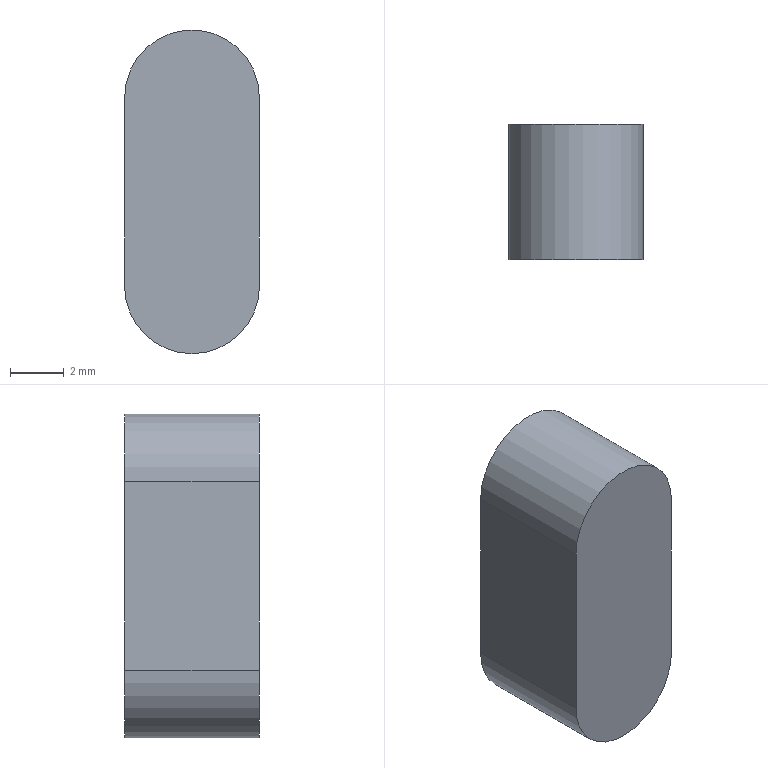Part | STEP file | BLC03-B5-L12 | 1 solid | 7 faces | box 5 x 5 x 12 mm | volume 273.175 mm3 | plane 4 | cylinder 3 | commonest cylinder face diameters 5 x3
STEP:
#1=CARTESIAN_POINT('',(0.,0.,0.));
#2=DIRECTION('',(0.,0.,1.));
#3=DIRECTION('',(1.,0.,0.));
#4=AXIS2_PLACEMENT_3D('',#1,#2,#3);
#5=CARTESIAN_POINT('',(0.,2.5,-6.));
#6=VERTEX_POINT('',#5);
#7=CARTESIAN_POINT('',(-2.5,2.5,-3.5));
#8=VERTEX_POINT('',#7);
#9=CARTESIAN_POINT('',(0.,2.5,-3.5));
#10=DIRECTION('',(0.,1.,0.));
#11=DIRECTION('',(0.,0.,1.));
#12=AXIS2_PLACEMENT_3D('',#9,#10,#11);
#13=CIRCLE('',#12,2.5);
#14=CARTESIAN_POINT('',(0.,2.5,-3.5));
#15=DIRECTION('',(0.,-1.,0.));
#16=DIRECTION('',(0.,0.,-1.));
#17=AXIS2_PLACEMENT_3D('',#14,#15,#16);
#18=CYLINDRICAL_SURFACE('',#17,2.5);
#19=CARTESIAN_POINT('',(9.425,0.));
#20=DIRECTION('',(-1.,0.));
#21=VECTOR('',#20,1.);
#22=LINE('',#19,#21);
#23=(GEOMETRIC_REPRESENTATION_CONTEXT(2)PARAMETRIC_REPRESENTATION_CONTEXT()REPRESENTATION_CONTEXT('',''));
#24=DEFINITIONAL_REPRESENTATION('',(#22),#23);
#25=PCURVE('',#18,#24);
#26=CARTESIAN_POINT('',(0.,2.5,3.5));
#27=DIRECTION('',(0.,1.,0.));
#28=DIRECTION('',(0.,0.,1.));
#29=AXIS2_PLACEMENT_3D('',#26,#27,#28);
#30=PLANE('',#29);
#31=CARTESIAN_POINT('',(-7.,0.));
#32=DIRECTION('',(1.,0.));
#33=AXIS2_PLACEMENT_2D('',#31,#32);
#34=CIRCLE('',#33,2.5);
#35=(GEOMETRIC_REPRESENTATION_CONTEXT(2)PARAMETRIC_REPRESENTATION_CONTEXT()REPRESENTATION_CONTEXT('',''));
#36=DEFINITIONAL_REPRESENTATION('',(#34),#35);
#37=PCURVE('',#30,#36);
#38=SURFACE_CURVE('',#13,(#25,#37),.PCURVE_S1.);
#39=EDGE_CURVE('',#6,#8,#38,.T.);
#40=ORIENTED_EDGE('',*,*,#39,.F.);
#41=CARTESIAN_POINT('',(0.,-2.5,-6.));
#42=VERTEX_POINT('',#41);
#43=CARTESIAN_POINT('',(0.,2.5,-6.));
#44=DIRECTION('',(0.,-1.,0.));
#45=VECTOR('',#44,1.);
#46=LINE('',#43,#45);
#47=CARTESIAN_POINT('',(6.283,0.));
#48=DIRECTION('',(0.,1.));
#49=VECTOR('',#48,1.);
#50=LINE('',#47,#49);
#51=(GEOMETRIC_REPRESENTATION_CONTEXT(2)PARAMETRIC_REPRESENTATION_CONTEXT()REPRESENTATION_CONTEXT('',''));
#52=DEFINITIONAL_REPRESENTATION('',(#50),#51);
#53=PCURVE('',#18,#52);
#54=CARTESIAN_POINT('',(0.,2.5,-3.5));
#55=DIRECTION('',(0.,-1.,0.));
#56=DIRECTION('',(0.,0.,-1.));
#57=AXIS2_PLACEMENT_3D('',#54,#55,#56);
#58=CYLINDRICAL_SURFACE('',#57,2.5);
#59=CARTESIAN_POINT('',(0.,0.));
#60=DIRECTION('',(0.,1.));
#61=VECTOR('',#60,1.);
#62=LINE('',#59,#61);
#63=(GEOMETRIC_REPRESENTATION_CONTEXT(2)PARAMETRIC_REPRESENTATION_CONTEXT()REPRESENTATION_CONTEXT('',''));
#64=DEFINITIONAL_REPRESENTATION('',(#62),#63);
#65=PCURVE('',#58,#64);
#66=SURFACE_CURVE('',#46,(#53,#65),.PCURVE_S1.);
#67=EDGE_CURVE('',#6,#42,#66,.T.);
#68=ORIENTED_EDGE('',*,*,#67,.T.);
#69=CARTESIAN_POINT('',(-2.5,-2.5,-3.5));
#70=VERTEX_POINT('',#69);
#71=CARTESIAN_POINT('',(0.,-2.5,-3.5));
#72=DIRECTION('',(0.,1.,0.));
#73=DIRECTION('',(0.,0.,1.));
#74=AXIS2_PLACEMENT_3D('',#71,#72,#73);
#75=CIRCLE('',#74,2.5);
#76=CARTESIAN_POINT('',(9.425,5.));
#77=DIRECTION('',(-1.,0.));
#78=VECTOR('',#77,1.);
#79=LINE('',#76,#78);
#80=(GEOMETRIC_REPRESENTATION_CONTEXT(2)PARAMETRIC_REPRESENTATION_CONTEXT()REPRESENTATION_CONTEXT('',''));
#81=DEFINITIONAL_REPRESENTATION('',(#79),#80);
#82=PCURVE('',#18,#81);
#83=CARTESIAN_POINT('',(0.,-2.5,3.5));
#84=DIRECTION('',(0.,1.,0.));
#85=DIRECTION('',(0.,0.,1.));
#86=AXIS2_PLACEMENT_3D('',#83,#84,#85);
#87=PLANE('',#86);
#88=CARTESIAN_POINT('',(-7.,0.));
#89=DIRECTION('',(1.,0.));
#90=AXIS2_PLACEMENT_2D('',#88,#89);
#91=CIRCLE('',#90,2.5);
#92=(GEOMETRIC_REPRESENTATION_CONTEXT(2)PARAMETRIC_REPRESENTATION_CONTEXT()REPRESENTATION_CONTEXT('',''));
#93=DEFINITIONAL_REPRESENTATION('',(#91),#92);
#94=PCURVE('',#87,#93);
#95=SURFACE_CURVE('',#75,(#82,#94),.PCURVE_S1.);
#96=EDGE_CURVE('',#42,#70,#95,.T.);
#97=ORIENTED_EDGE('',*,*,#96,.T.);
#98=CARTESIAN_POINT('',(-2.5,2.5,-3.5));
#99=DIRECTION('',(0.,-1.,0.));
#100=VECTOR('',#99,1.);
#101=LINE('',#98,#100);
#102=CARTESIAN_POINT('',(4.712,0.));
#103=DIRECTION('',(0.,1.));
#104=VECTOR('',#103,1.);
#105=LINE('',#102,#104);
#106=(GEOMETRIC_REPRESENTATION_CONTEXT(2)PARAMETRIC_REPRESENTATION_CONTEXT()REPRESENTATION_CONTEXT('',''));
#107=DEFINITIONAL_REPRESENTATION('',(#105),#106);
#108=PCURVE('',#18,#107);
#109=CARTESIAN_POINT('',(-2.5,2.5,-3.5));
#110=DIRECTION('',(1.,0.,0.));
#111=DIRECTION('',(0.,0.,-1.));
#112=AXIS2_PLACEMENT_3D('',#109,#110,#111);
#113=PLANE('',#112);
#114=CARTESIAN_POINT('',(0.,0.));
#115=DIRECTION('',(0.,-1.));
#116=VECTOR('',#115,1.);
#117=LINE('',#114,#116);
#118=(GEOMETRIC_REPRESENTATION_CONTEXT(2)PARAMETRIC_REPRESENTATION_CONTEXT()REPRESENTATION_CONTEXT('',''));
#119=DEFINITIONAL_REPRESENTATION('',(#117),#118);
#120=PCURVE('',#113,#119);
#121=SURFACE_CURVE('',#101,(#108,#120),.PCURVE_S1.);
#122=EDGE_CURVE('',#8,#70,#121,.T.);
#123=ORIENTED_EDGE('',*,*,#122,.F.);
#124=EDGE_LOOP('',(#40,#68,#97,#123));
#125=FACE_BOUND('',#124,.T.);
#126=ADVANCED_FACE('',(#125),#18,.T.);
#127=CARTESIAN_POINT('',(2.5,-2.5,-3.5));
#128=VERTEX_POINT('',#127);
#129=CARTESIAN_POINT('',(2.5,-2.5,3.5));
#130=VERTEX_POINT('',#129);
#131=CARTESIAN_POINT('',(2.5,-2.5,-3.5));
#132=DIRECTION('',(0.,0.,1.));
#133=VECTOR('',#132,1.);
#134=LINE('',#131,#133);
#135=CARTESIAN_POINT('',(2.5,2.5,-3.5));
#136=DIRECTION('',(1.,0.,0.));
#137=DIRECTION('',(0.,0.,-1.));
#138=AXIS2_PLACEMENT_3D('',#135,#136,#137);
#139=PLANE('',#138);
#140=CARTESIAN_POINT('',(0.,-5.));
#141=DIRECTION('',(-1.,0.));
#142=VECTOR('',#141,1.);
#143=LINE('',#140,#142);
#144=(GEOMETRIC_REPRESENTATION_CONTEXT(2)PARAMETRIC_REPRESENTATION_CONTEXT()REPRESENTATION_CONTEXT('',''));
#145=DEFINITIONAL_REPRESENTATION('',(#143),#144);
#146=PCURVE('',#139,#145);
#147=CARTESIAN_POINT('',(-7.,2.5));
#148=DIRECTION('',(1.,0.));
#149=VECTOR('',#148,1.);
#150=LINE('',#147,#149);
#151=(GEOMETRIC_REPRESENTATION_CONTEXT(2)PARAMETRIC_REPRESENTATION_CONTEXT()REPRESENTATION_CONTEXT('',''));
#152=DEFINITIONAL_REPRESENTATION('',(#150),#151);
#153=PCURVE('',#87,#152);
#154=SURFACE_CURVE('',#134,(#146,#153),.PCURVE_S1.);
#155=EDGE_CURVE('',#128,#130,#154,.T.);
#156=ORIENTED_EDGE('',*,*,#155,.F.);
#157=CARTESIAN_POINT('',(2.5,2.5,-3.5));
#158=VERTEX_POINT('',#157);
#159=CARTESIAN_POINT('',(2.5,2.5,-3.5));
#160=DIRECTION('',(0.,-1.,0.));
#161=VECTOR('',#160,1.);
#162=LINE('',#159,#161);
#163=CARTESIAN_POINT('',(0.,0.));
#164=DIRECTION('',(0.,-1.));
#165=VECTOR('',#164,1.);
#166=LINE('',#163,#165);
#167=(GEOMETRIC_REPRESENTATION_CONTEXT(2)PARAMETRIC_REPRESENTATION_CONTEXT()REPRESENTATION_CONTEXT('',''));
#168=DEFINITIONAL_REPRESENTATION('',(#166),#167);
#169=PCURVE('',#139,#168);
#170=CARTESIAN_POINT('',(1.571,0.));
#171=DIRECTION('',(0.,1.));
#172=VECTOR('',#171,1.);
#173=LINE('',#170,#172);
#174=(GEOMETRIC_REPRESENTATION_CONTEXT(2)PARAMETRIC_REPRESENTATION_CONTEXT()REPRESENTATION_CONTEXT('',''));
#175=DEFINITIONAL_REPRESENTATION('',(#173),#174);
#176=PCURVE('',#58,#175);
#177=SURFACE_CURVE('',#162,(#169,#176),.PCURVE_S1.);
#178=EDGE_CURVE('',#158,#128,#177,.T.);
#179=ORIENTED_EDGE('',*,*,#178,.F.);
#180=CARTESIAN_POINT('',(2.5,2.5,3.5));
#181=VERTEX_POINT('',#180);
#182=CARTESIAN_POINT('',(2.5,2.5,-3.5));
#183=DIRECTION('',(0.,0.,1.));
#184=VECTOR('',#183,1.);
#185=LINE('',#182,#184);
#186=CARTESIAN_POINT('',(0.,0.));
#187=DIRECTION('',(-1.,0.));
#188=VECTOR('',#187,1.);
#189=LINE('',#186,#188);
#190=(GEOMETRIC_REPRESENTATION_CONTEXT(2)PARAMETRIC_REPRESENTATION_CONTEXT()REPRESENTATION_CONTEXT('',''));
#191=DEFINITIONAL_REPRESENTATION('',(#189),#190);
#192=PCURVE('',#139,#191);
#193=CARTESIAN_POINT('',(-7.,2.5));
#194=DIRECTION('',(1.,0.));
#195=VECTOR('',#194,1.);
#196=LINE('',#193,#195);
#197=(GEOMETRIC_REPRESENTATION_CONTEXT(2)PARAMETRIC_REPRESENTATION_CONTEXT()REPRESENTATION_CONTEXT('',''));
#198=DEFINITIONAL_REPRESENTATION('',(#196),#197);
#199=PCURVE('',#30,#198);
#200=SURFACE_CURVE('',#185,(#192,#199),.PCURVE_S1.);
#201=EDGE_CURVE('',#158,#181,#200,.T.);
#202=ORIENTED_EDGE('',*,*,#201,.T.);
#203=CARTESIAN_POINT('',(2.5,2.5,3.5));
#204=DIRECTION('',(0.,-1.,0.));
#205=VECTOR('',#204,1.);
#206=LINE('',#203,#205);
#207=CARTESIAN_POINT('',(-7.,0.));
#208=DIRECTION('',(0.,-1.));
#209=VECTOR('',#208,1.);
#210=LINE('',#207,#209);
#211=(GEOMETRIC_REPRESENTATION_CONTEXT(2)PARAMETRIC_REPRESENTATION_CONTEXT()REPRESENTATION_CONTEXT('',''));
#212=DEFINITIONAL_REPRESENTATION('',(#210),#211);
#213=PCURVE('',#139,#212);
#214=CARTESIAN_POINT('',(0.,2.5,3.5));
#215=DIRECTION('',(0.,-1.,0.));
#216=DIRECTION('',(0.,0.,-1.));
#217=AXIS2_PLACEMENT_3D('',#214,#215,#216);
#218=CYLINDRICAL_SURFACE('',#217,2.5);
#219=CARTESIAN_POINT('',(1.571,0.));
#220=DIRECTION('',(0.,1.));
#221=VECTOR('',#220,1.);
#222=LINE('',#219,#221);
#223=(GEOMETRIC_REPRESENTATION_CONTEXT(2)PARAMETRIC_REPRESENTATION_CONTEXT()REPRESENTATION_CONTEXT('',''));
#224=DEFINITIONAL_REPRESENTATION('',(#222),#223);
#225=PCURVE('',#218,#224);
#226=SURFACE_CURVE('',#206,(#213,#225),.PCURVE_S1.);
#227=EDGE_CURVE('',#181,#130,#226,.T.);
#228=ORIENTED_EDGE('',*,*,#227,.T.);
#229=EDGE_LOOP('',(#156,#179,#202,#228));
#230=FACE_BOUND('',#229,.T.);
#231=ADVANCED_FACE('',(#230),#139,.T.);
#232=ORIENTED_EDGE('',*,*,#67,.F.);
#233=CARTESIAN_POINT('',(0.,2.5,-3.5));
#234=DIRECTION('',(0.,1.,0.));
#235=DIRECTION('',(0.,0.,1.));
#236=AXIS2_PLACEMENT_3D('',#233,#234,#235);
#237=CIRCLE('',#236,2.5);
#238=CARTESIAN_POINT('',(3.142,0.));
#239=DIRECTION('',(-1.,0.));
#240=VECTOR('',#239,1.);
#241=LINE('',#238,#240);
#242=(GEOMETRIC_REPRESENTATION_CONTEXT(2)PARAMETRIC_REPRESENTATION_CONTEXT()REPRESENTATION_CONTEXT('',''));
#243=DEFINITIONAL_REPRESENTATION('',(#241),#242);
#244=PCURVE('',#58,#243);
#245=CARTESIAN_POINT('',(-7.,0.));
#246=DIRECTION('',(1.,0.));
#247=AXIS2_PLACEMENT_2D('',#245,#246);
#248=CIRCLE('',#247,2.5);
#249=(GEOMETRIC_REPRESENTATION_CONTEXT(2)PARAMETRIC_REPRESENTATION_CONTEXT()REPRESENTATION_CONTEXT('',''));
#250=DEFINITIONAL_REPRESENTATION('',(#248),#249);
#251=PCURVE('',#30,#250);
#252=SURFACE_CURVE('',#237,(#244,#251),.PCURVE_S1.);
#253=EDGE_CURVE('',#158,#6,#252,.T.);
#254=ORIENTED_EDGE('',*,*,#253,.F.);
#255=ORIENTED_EDGE('',*,*,#178,.T.);
#256=CARTESIAN_POINT('',(0.,-2.5,-3.5));
#257=DIRECTION('',(0.,1.,0.));
#258=DIRECTION('',(0.,0.,1.));
#259=AXIS2_PLACEMENT_3D('',#256,#257,#258);
#260=CIRCLE('',#259,2.5);
#261=CARTESIAN_POINT('',(3.142,5.));
#262=DIRECTION('',(-1.,0.));
#263=VECTOR('',#262,1.);
#264=LINE('',#261,#263);
#265=(GEOMETRIC_REPRESENTATION_CONTEXT(2)PARAMETRIC_REPRESENTATION_CONTEXT()REPRESENTATION_CONTEXT('',''));
#266=DEFINITIONAL_REPRESENTATION('',(#264),#265);
#267=PCURVE('',#58,#266);
#268=CARTESIAN_POINT('',(-7.,0.));
#269=DIRECTION('',(1.,0.));
#270=AXIS2_PLACEMENT_2D('',#268,#269);
#271=CIRCLE('',#270,2.5);
#272=(GEOMETRIC_REPRESENTATION_CONTEXT(2)PARAMETRIC_REPRESENTATION_CONTEXT()REPRESENTATION_CONTEXT('',''));
#273=DEFINITIONAL_REPRESENTATION('',(#271),#272);
#274=PCURVE('',#87,#273);
#275=SURFACE_CURVE('',#260,(#267,#274),.PCURVE_S1.);
#276=EDGE_CURVE('',#128,#42,#275,.T.);
#277=ORIENTED_EDGE('',*,*,#276,.T.);
#278=EDGE_LOOP('',(#232,#254,#255,#277));
#279=FACE_BOUND('',#278,.T.);
#280=ADVANCED_FACE('',(#279),#58,.T.);
#281=CARTESIAN_POINT('',(-2.5,-2.5,3.5));
#282=VERTEX_POINT('',#281);
#283=CARTESIAN_POINT('',(-2.5,-2.5,-3.5));
#284=DIRECTION('',(0.,0.,1.));
#285=VECTOR('',#284,1.);
#286=LINE('',#283,#285);
#287=CARTESIAN_POINT('',(0.,-5.));
#288=DIRECTION('',(-1.,0.));
#289=VECTOR('',#288,1.);
#290=LINE('',#287,#289);
#291=(GEOMETRIC_REPRESENTATION_CONTEXT(2)PARAMETRIC_REPRESENTATION_CONTEXT()REPRESENTATION_CONTEXT('',''));
#292=DEFINITIONAL_REPRESENTATION('',(#290),#291);
#293=PCURVE('',#113,#292);
#294=CARTESIAN_POINT('',(-7.,-2.5));
#295=DIRECTION('',(1.,0.));
#296=VECTOR('',#295,1.);
#297=LINE('',#294,#296);
#298=(GEOMETRIC_REPRESENTATION_CONTEXT(2)PARAMETRIC_REPRESENTATION_CONTEXT()REPRESENTATION_CONTEXT('',''));
#299=DEFINITIONAL_REPRESENTATION('',(#297),#298);
#300=PCURVE('',#87,#299);
#301=SURFACE_CURVE('',#286,(#293,#300),.PCURVE_S1.);
#302=EDGE_CURVE('',#70,#282,#301,.T.);
#303=ORIENTED_EDGE('',*,*,#302,.T.);
#304=CARTESIAN_POINT('',(-2.5,2.5,3.5));
#305=VERTEX_POINT('',#304);
#306=CARTESIAN_POINT('',(-2.5,2.5,3.5));
#307=DIRECTION('',(0.,-1.,0.));
#308=VECTOR('',#307,1.);
#309=LINE('',#306,#308);
#310=CARTESIAN_POINT('',(-7.,0.));
#311=DIRECTION('',(0.,-1.));
#312=VECTOR('',#311,1.);
#313=LINE('',#310,#312);
#314=(GEOMETRIC_REPRESENTATION_CONTEXT(2)PARAMETRIC_REPRESENTATION_CONTEXT()REPRESENTATION_CONTEXT('',''));
#315=DEFINITIONAL_REPRESENTATION('',(#313),#314);
#316=PCURVE('',#113,#315);
#317=CARTESIAN_POINT('',(4.712,0.));
#318=DIRECTION('',(0.,1.));
#319=VECTOR('',#318,1.);
#320=LINE('',#317,#319);
#321=(GEOMETRIC_REPRESENTATION_CONTEXT(2)PARAMETRIC_REPRESENTATION_CONTEXT()REPRESENTATION_CONTEXT('',''));
#322=DEFINITIONAL_REPRESENTATION('',(#320),#321);
#323=PCURVE('',#218,#322);
#324=SURFACE_CURVE('',#309,(#316,#323),.PCURVE_S1.);
#325=EDGE_CURVE('',#305,#282,#324,.T.);
#326=ORIENTED_EDGE('',*,*,#325,.F.);
#327=CARTESIAN_POINT('',(-2.5,2.5,-3.5));
#328=DIRECTION('',(0.,0.,1.));
#329=VECTOR('',#328,1.);
#330=LINE('',#327,#329);
#331=CARTESIAN_POINT('',(0.,0.));
#332=DIRECTION('',(-1.,0.));
#333=VECTOR('',#332,1.);
#334=LINE('',#331,#333);
#335=(GEOMETRIC_REPRESENTATION_CONTEXT(2)PARAMETRIC_REPRESENTATION_CONTEXT()REPRESENTATION_CONTEXT('',''));
#336=DEFINITIONAL_REPRESENTATION('',(#334),#335);
#337=PCURVE('',#113,#336);
#338=CARTESIAN_POINT('',(-7.,-2.5));
#339=DIRECTION('',(1.,0.));
#340=VECTOR('',#339,1.);
#341=LINE('',#338,#340);
#342=(GEOMETRIC_REPRESENTATION_CONTEXT(2)PARAMETRIC_REPRESENTATION_CONTEXT()REPRESENTATION_CONTEXT('',''));
#343=DEFINITIONAL_REPRESENTATION('',(#341),#342);
#344=PCURVE('',#30,#343);
#345=SURFACE_CURVE('',#330,(#337,#344),.PCURVE_S1.);
#346=EDGE_CURVE('',#8,#305,#345,.T.);
#347=ORIENTED_EDGE('',*,*,#346,.F.);
#348=ORIENTED_EDGE('',*,*,#122,.T.);
#349=EDGE_LOOP('',(#303,#326,#347,#348));
#350=FACE_BOUND('',#349,.T.);
#351=ADVANCED_FACE('',(#350),#113,.F.);
#352=CARTESIAN_POINT('',(0.,-2.5,3.5));
#353=DIRECTION('',(0.,1.,0.));
#354=DIRECTION('',(0.,0.,1.));
#355=AXIS2_PLACEMENT_3D('',#352,#353,#354);
#356=CIRCLE('',#355,2.5);
#357=CARTESIAN_POINT('',(9.425,5.));
#358=DIRECTION('',(-1.,0.));
#359=VECTOR('',#358,1.);
#360=LINE('',#357,#359);
#361=(GEOMETRIC_REPRESENTATION_CONTEXT(2)PARAMETRIC_REPRESENTATION_CONTEXT()REPRESENTATION_CONTEXT('',''));
#362=DEFINITIONAL_REPRESENTATION('',(#360),#361);
#363=PCURVE('',#218,#362);
#364=CARTESIAN_POINT('',(0.,0.));
#365=DIRECTION('',(1.,0.));
#366=AXIS2_PLACEMENT_2D('',#364,#365);
#367=CIRCLE('',#366,2.5);
#368=(GEOMETRIC_REPRESENTATION_CONTEXT(2)PARAMETRIC_REPRESENTATION_CONTEXT()REPRESENTATION_CONTEXT('',''));
#369=DEFINITIONAL_REPRESENTATION('',(#367),#368);
#370=PCURVE('',#87,#369);
#371=SURFACE_CURVE('',#356,(#363,#370),.PCURVE_S1.);
#372=EDGE_CURVE('',#282,#130,#371,.T.);
#373=ORIENTED_EDGE('',*,*,#372,.T.);
#374=ORIENTED_EDGE('',*,*,#227,.F.);
#375=CARTESIAN_POINT('',(0.,2.5,3.5));
#376=DIRECTION('',(0.,1.,0.));
#377=DIRECTION('',(0.,0.,1.));
#378=AXIS2_PLACEMENT_3D('',#375,#376,#377);
#379=CIRCLE('',#378,2.5);
#380=CARTESIAN_POINT('',(9.425,0.));
#381=DIRECTION('',(-1.,0.));
#382=VECTOR('',#381,1.);
#383=LINE('',#380,#382);
#384=(GEOMETRIC_REPRESENTATION_CONTEXT(2)PARAMETRIC_REPRESENTATION_CONTEXT()REPRESENTATION_CONTEXT('',''));
#385=DEFINITIONAL_REPRESENTATION('',(#383),#384);
#386=PCURVE('',#218,#385);
#387=CARTESIAN_POINT('',(0.,0.));
#388=DIRECTION('',(1.,0.));
#389=AXIS2_PLACEMENT_2D('',#387,#388);
#390=CIRCLE('',#389,2.5);
#391=(GEOMETRIC_REPRESENTATION_CONTEXT(2)PARAMETRIC_REPRESENTATION_CONTEXT()REPRESENTATION_CONTEXT('',''));
#392=DEFINITIONAL_REPRESENTATION('',(#390),#391);
#393=PCURVE('',#30,#392);
#394=SURFACE_CURVE('',#379,(#386,#393),.PCURVE_S1.);
#395=EDGE_CURVE('',#305,#181,#394,.T.);
#396=ORIENTED_EDGE('',*,*,#395,.F.);
#397=ORIENTED_EDGE('',*,*,#325,.T.);
#398=EDGE_LOOP('',(#373,#374,#396,#397));
#399=FACE_BOUND('',#398,.T.);
#400=ADVANCED_FACE('',(#399),#218,.T.);
#401=ORIENTED_EDGE('',*,*,#201,.F.);
#402=ORIENTED_EDGE('',*,*,#253,.T.);
#403=ORIENTED_EDGE('',*,*,#39,.T.);
#404=ORIENTED_EDGE('',*,*,#346,.T.);
#405=ORIENTED_EDGE('',*,*,#395,.T.);
#406=EDGE_LOOP('',(#401,#402,#403,#404,#405));
#407=FACE_BOUND('',#406,.T.);
#408=ADVANCED_FACE('',(#407),#30,.T.);
#409=ORIENTED_EDGE('',*,*,#155,.T.);
#410=ORIENTED_EDGE('',*,*,#372,.F.);
#411=ORIENTED_EDGE('',*,*,#302,.F.);
#412=ORIENTED_EDGE('',*,*,#96,.F.);
#413=ORIENTED_EDGE('',*,*,#276,.F.);
#414=EDGE_LOOP('',(#409,#410,#411,#412,#413));
#415=FACE_BOUND('',#414,.T.);
#416=ADVANCED_FACE('',(#415),#87,.F.);
#417=CLOSED_SHELL('',(#126,#231,#280,#351,#400,#408,#416));
#418=MANIFOLD_SOLID_BREP('',#417);
#419=(LENGTH_UNIT()NAMED_UNIT(*)SI_UNIT(.MILLI.,.METRE.));
#420=UNCERTAINTY_MEASURE_WITH_UNIT(LENGTH_MEASURE(0.0000001),#419,'','');
#421=(NAMED_UNIT(*)PLANE_ANGLE_UNIT()SI_UNIT($,.RADIAN.));
#422=(NAMED_UNIT(*)SI_UNIT($,.STERADIAN.)SOLID_ANGLE_UNIT());
#423=(GEOMETRIC_REPRESENTATION_CONTEXT(3)GLOBAL_UNCERTAINTY_ASSIGNED_CONTEXT((#420))GLOBAL_UNIT_ASSIGNED_CONTEXT((#419,#421,#422))REPRESENTATION_CONTEXT('',''));
#424=ADVANCED_BREP_SHAPE_REPRESENTATION('',(#4,#418),#423);